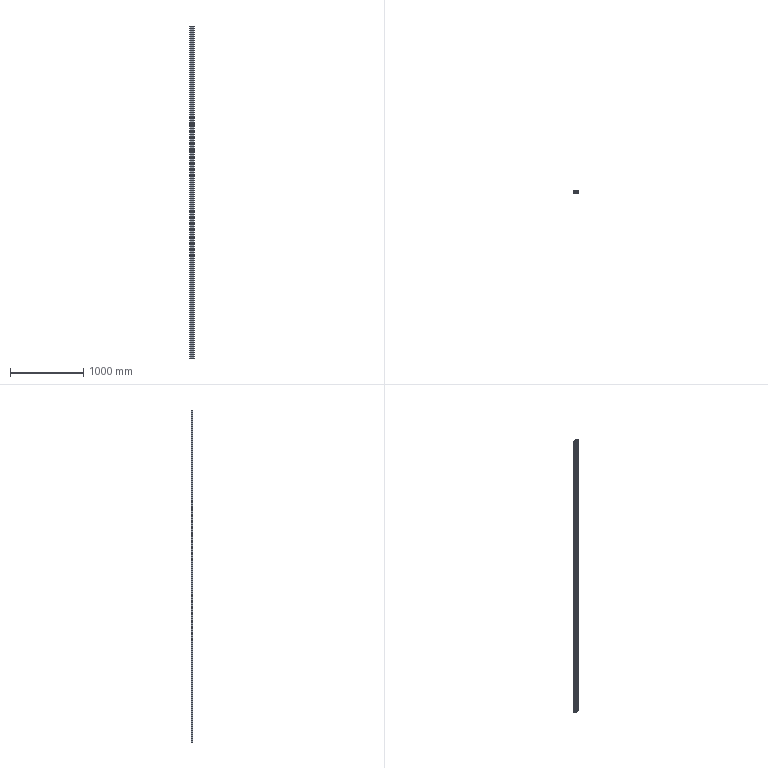Part | SolidWorks | features MBimport 1, MoveFace 1 | 1 solid | 168 faces | box 60 x 20 x 4546 mm | volume 1925976 mm3 | plane 142 | cylinder 26 | commonest cylinder face diameters 0.4 x16 5 x6 3 x4